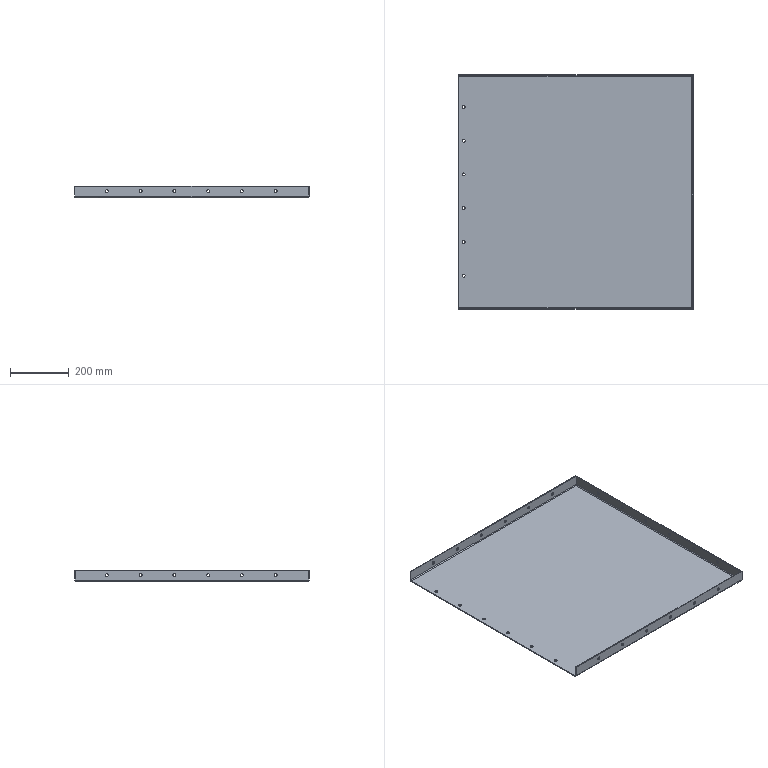Part | SolidWorks | features ICE 3, CornerFeat 2, EdgeFlange 2, FlatPattern 1, SMBaseFlange 1, SheetMetal 1 | 1 solid | 78 faces | box 800 x 800 x 40 mm | volume 2166122 mm3 | cylinder 54 | plane 20 | spline 4 | commonest cylinder face diameters 10 x48 6 x3 12 x3